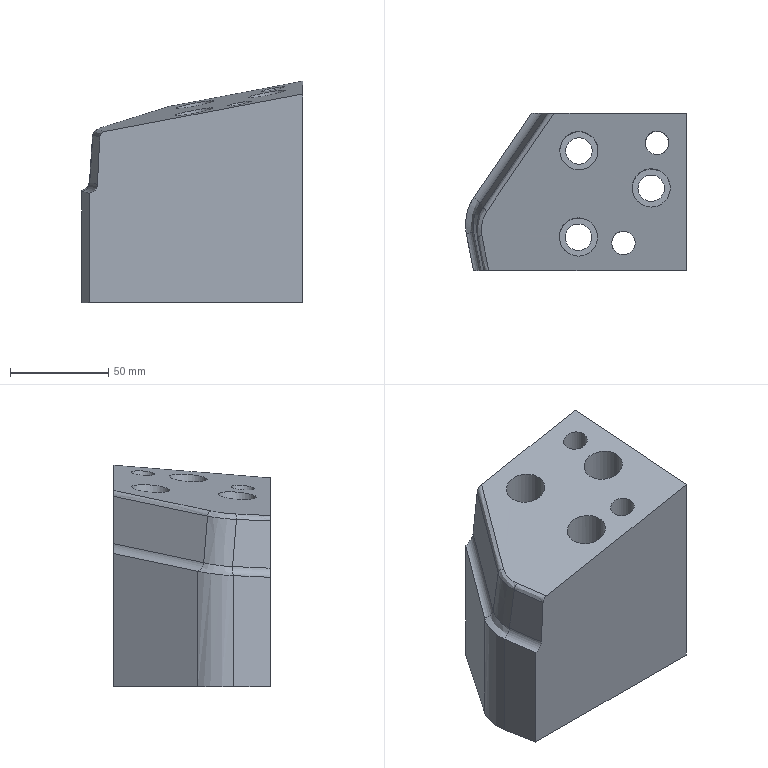Part | NX | features solid 2 | 1 solid | 28 faces | box 112.653 x 80 x 112.905 mm | volume 689812 mm3 | cylinder 10 | spline 9 | plane 9 | commonest cylinder face diameters 13.5 x3 19.5 x3 10 x2 12 x2
STEP:
#1=CARTESIAN_POINT('',(910.176,4.689,67.517));
#2=VERTEX_POINT('',#1);
#3=CARTESIAN_POINT('',(904.312,-0.5268,65.98));
#4=CARTESIAN_POINT('',(911.039,4.097,67.632));
#5=CARTESIAN_POINT('',(912.591,12.271,68.592));
#6=CARTESIAN_POINT('',(907.787,19.138,68.239));
#7=CARTESIAN_POINT('',(899.676,20.525,66.813));
#8=CARTESIAN_POINT('',(892.968,15.903,65.165));
#9=CARTESIAN_POINT('',(891.404,7.747,64.204));
#10=CARTESIAN_POINT('',(896.213,0.8606,64.556));
#11=CARTESIAN_POINT('',(904.312,-0.5268,65.98));
#12=CARTESIAN_POINT('',(911.039,4.097,67.632));
#13=CARTESIAN_POINT('',(912.591,12.271,68.592));
#14=B_SPLINE_CURVE_WITH_KNOTS('',3,(#3,#4,#5,#6,#7,#8,#9,#10,#11,#12,#13),.UNSPECIFIED.,.T.,.F.,(1,1,1,1,1,1,1,1,1,1,1,1,1,1,1),(-0.0231,-0.0154,-0.007701,0.,0.007701,0.0154,0.0231,0.0308,0.03851,0.04621,0.05391,0.06161,0.06931,0.07701,0.08471),.UNSPECIFIED.);
#15=EDGE_CURVE('',#2,#2,#14,.T.);
#16=ORIENTED_EDGE('',*,*,#15,.F.);
#17=EDGE_LOOP('',(#16));
#18=FACE_BOUND('',#17,.T.);
#19=CARTESIAN_POINT('',(874.601,-16.091,59.076));
#20=VERTEX_POINT('',#19);
#21=CARTESIAN_POINT('',(871.629,-23.43,57.915));
#22=CARTESIAN_POINT('',(875.665,-16.236,59.267));
#23=CARTESIAN_POINT('',(873.318,-8.171,59.478));
#24=CARTESIAN_POINT('',(866.002,-4.266,58.407));
#25=CARTESIAN_POINT('',(858.186,-6.577,56.737));
#26=CARTESIAN_POINT('',(854.166,-13.76,55.389));
#27=CARTESIAN_POINT('',(856.494,-21.817,55.175));
#28=CARTESIAN_POINT('',(863.825,-25.735,56.247));
#29=CARTESIAN_POINT('',(871.629,-23.43,57.915));
#30=CARTESIAN_POINT('',(875.665,-16.236,59.267));
#31=CARTESIAN_POINT('',(873.318,-8.171,59.478));
#32=B_SPLINE_CURVE_WITH_KNOTS('',3,(#21,#22,#23,#24,#25,#26,#27,#28,#29,#30,#31),.UNSPECIFIED.,.T.,.F.,(1,1,1,1,1,1,1,1,1,1,1,1,1,1,1),(-0.02311,-0.0154,-0.007702,0.,0.007702,0.0154,0.02311,0.03081,0.03851,0.04621,0.05392,0.06162,0.06932,0.07702,0.08472),.UNSPECIFIED.);
#33=EDGE_CURVE('',#20,#20,#32,.T.);
#34=ORIENTED_EDGE('',*,*,#33,.F.);
#35=EDGE_LOOP('',(#34));
#36=FACE_BOUND('',#35,.T.);
#37=CARTESIAN_POINT('',(874.42,25.901,62.459));
#38=VERTEX_POINT('',#37);
#39=CARTESIAN_POINT('',(870.01,19.371,61.091));
#40=CARTESIAN_POINT('',(875.417,25.536,62.619));
#41=CARTESIAN_POINT('',(874.842,33.891,63.19));
#42=CARTESIAN_POINT('',(868.479,39.284,62.421));
#43=CARTESIAN_POINT('',(860.329,38.624,60.821));
#44=CARTESIAN_POINT('',(854.941,32.466,59.298));
#45=CARTESIAN_POINT('',(855.498,24.125,58.725));
#46=CARTESIAN_POINT('',(861.874,18.715,59.494));
#47=CARTESIAN_POINT('',(870.01,19.371,61.091));
#48=CARTESIAN_POINT('',(875.417,25.536,62.619));
#49=CARTESIAN_POINT('',(874.842,33.891,63.19));
#50=B_SPLINE_CURVE_WITH_KNOTS('',3,(#39,#40,#41,#42,#43,#44,#45,#46,#47,#48,#49),.UNSPECIFIED.,.T.,.F.,(1,1,1,1,1,1,1,1,1,1,1,1,1,1,1),(-0.02311,-0.0154,-0.007702,0.,0.007702,0.0154,0.02311,0.03081,0.03851,0.04621,0.05391,0.06162,0.06932,0.07702,0.08472),.UNSPECIFIED.);
#51=EDGE_CURVE('',#38,#38,#50,.T.);
#52=ORIENTED_EDGE('',*,*,#51,.F.);
#53=EDGE_LOOP('',(#52));
#54=FACE_BOUND('',#53,.T.);
#55=CARTESIAN_POINT('',(900.381,36.794,68.271));
#56=VERTEX_POINT('',#55);
#57=CARTESIAN_POINT('',(904.331,39.565,69.246));
#58=CARTESIAN_POINT('',(899.898,37.213,68.213));
#59=CARTESIAN_POINT('',(898.365,32.347,67.527));
#60=CARTESIAN_POINT('',(900.8,27.795,67.618));
#61=CARTESIAN_POINT('',(905.676,26.363,68.427));
#62=CARTESIAN_POINT('',(910.098,28.715,69.457));
#63=CARTESIAN_POINT('',(911.636,33.57,70.144));
#64=CARTESIAN_POINT('',(909.201,38.133,70.053));
#65=CARTESIAN_POINT('',(904.331,39.565,69.246));
#66=CARTESIAN_POINT('',(899.898,37.213,68.213));
#67=CARTESIAN_POINT('',(898.365,32.347,67.527));
#68=B_SPLINE_CURVE_WITH_KNOTS('',3,(#57,#58,#59,#60,#61,#62,#63,#64,#65,#66,#67),.UNSPECIFIED.,.T.,.F.,(1,1,1,1,1,1,1,1,1,1,1,1,1,1,1),(-0.01422,-0.009478,-0.004739,0.,0.004739,0.009478,0.01422,0.01896,0.02369,0.02843,0.03317,0.03791,0.04265,0.04739,0.05213),.UNSPECIFIED.);
#69=EDGE_CURVE('',#56,#56,#68,.T.);
#70=ORIENTED_EDGE('',*,*,#69,.F.);
#71=EDGE_LOOP('',(#70));
#72=FACE_BOUND('',#71,.T.);
#73=CARTESIAN_POINT('',(818.332,-1.794,49.565));
#74=VERTEX_POINT('',#73);
#75=CARTESIAN_POINT('',(815.743,-14.303,48.056));
#76=VERTEX_POINT('',#75);
#77=CARTESIAN_POINT('',(818.332,-1.794,49.565));
#78=CARTESIAN_POINT('',(815.864,-5.396,48.803));
#79=CARTESIAN_POINT('',(814.905,-9.954,48.251));
#80=CARTESIAN_POINT('',(815.743,-14.303,48.056));
#81=B_SPLINE_CURVE_WITH_KNOTS('',3,(#77,#78,#79,#80),.UNSPECIFIED.,.F.,.F.,(4,4),(0.,0.01319),.UNSPECIFIED.);
#82=EDGE_CURVE('',#74,#76,#81,.T.);
#83=ORIENTED_EDGE('',*,*,#82,.T.);
#84=CARTESIAN_POINT('',(819.154,-32.,47.263));
#85=VERTEX_POINT('',#84);
#86=CARTESIAN_POINT('',(815.743,-14.303,48.056));
#87=CARTESIAN_POINT('',(816.88,-20.202,47.791));
#88=CARTESIAN_POINT('',(818.017,-26.101,47.527));
#89=CARTESIAN_POINT('',(819.154,-32.,47.263));
#90=B_SPLINE_CURVE_WITH_KNOTS('',3,(#86,#87,#88,#89),.UNSPECIFIED.,.F.,.F.,(4,4),(0.,0.01804),.UNSPECIFIED.);
#91=EDGE_CURVE('',#76,#85,#90,.T.);
#92=ORIENTED_EDGE('',*,*,#91,.T.);
#93=CARTESIAN_POINT('',(920.,-32.,66.395));
#94=VERTEX_POINT('',#93);
#95=CARTESIAN_POINT('',(819.154,-32.,47.263));
#96=CARTESIAN_POINT('',(852.769,-32.,53.64));
#97=CARTESIAN_POINT('',(886.385,-32.,60.017));
#98=CARTESIAN_POINT('',(920.,-32.,66.395));
#99=B_SPLINE_CURVE_WITH_KNOTS('',3,(#95,#96,#97,#98),.UNSPECIFIED.,.F.,.F.,(4,4),(0.,0.1026),.UNSPECIFIED.);
#100=EDGE_CURVE('',#85,#94,#99,.T.);
#101=ORIENTED_EDGE('',*,*,#100,.T.);
#102=CARTESIAN_POINT('',(920.,48.,72.905));
#103=VERTEX_POINT('',#102);
#104=CARTESIAN_POINT('',(920.,-32.,66.395));
#105=CARTESIAN_POINT('',(920.,-5.333,68.565));
#106=CARTESIAN_POINT('',(920.,21.333,70.735));
#107=CARTESIAN_POINT('',(920.,48.,72.905));
#108=B_SPLINE_CURVE_WITH_KNOTS('',3,(#104,#105,#106,#107),.UNSPECIFIED.,.F.,.F.,(4,4),(0.,0.08026),.UNSPECIFIED.);
#109=EDGE_CURVE('',#94,#103,#108,.T.);
#110=ORIENTED_EDGE('',*,*,#109,.T.);
#111=CARTESIAN_POINT('',(852.448,48.,60.089));
#112=VERTEX_POINT('',#111);
#113=CARTESIAN_POINT('',(852.448,48.,60.089));
#114=CARTESIAN_POINT('',(874.965,48.,64.361));
#115=CARTESIAN_POINT('',(897.483,48.,68.633));
#116=CARTESIAN_POINT('',(920.,48.,72.905));
#117=B_SPLINE_CURVE_WITH_KNOTS('',3,(#113,#114,#115,#116),.UNSPECIFIED.,.F.,.F.,(4,4),(0.,0.06876),.UNSPECIFIED.);
#118=EDGE_CURVE('',#112,#103,#117,.T.);
#119=ORIENTED_EDGE('',*,*,#118,.F.);
#120=CARTESIAN_POINT('',(852.448,48.,60.089));
#121=CARTESIAN_POINT('',(841.076,31.402,56.581));
#122=CARTESIAN_POINT('',(829.704,14.804,53.073));
#123=CARTESIAN_POINT('',(818.332,-1.794,49.565));
#124=B_SPLINE_CURVE_WITH_KNOTS('',3,(#120,#121,#122,#123),.UNSPECIFIED.,.F.,.F.,(4,4),(0.0001037,0.06137),.UNSPECIFIED.);
#125=EDGE_CURVE('',#112,#74,#124,.T.);
#126=ORIENTED_EDGE('',*,*,#125,.T.);
#127=EDGE_LOOP('',(#83,#92,#101,#110,#119,#126));
#128=FACE_BOUND('',#127,.T.);
#129=CARTESIAN_POINT('',(882.556,-15.206,60.658));
#130=VERTEX_POINT('',#129);
#131=CARTESIAN_POINT('',(885.863,-11.678,61.572));
#132=CARTESIAN_POINT('',(881.991,-14.889,60.576));
#133=CARTESIAN_POINT('',(881.506,-20.,60.068));
#134=CARTESIAN_POINT('',(884.84,-23.925,60.381));
#135=CARTESIAN_POINT('',(889.875,-24.32,61.305));
#136=CARTESIAN_POINT('',(893.735,-21.111,62.298));
#137=CARTESIAN_POINT('',(894.229,-16.011,62.807));
#138=CARTESIAN_POINT('',(890.89,-12.074,62.494));
#139=CARTESIAN_POINT('',(885.863,-11.678,61.572));
#140=CARTESIAN_POINT('',(881.991,-14.889,60.576));
#141=CARTESIAN_POINT('',(881.506,-20.,60.068));
#142=B_SPLINE_CURVE_WITH_KNOTS('',3,(#131,#132,#133,#134,#135,#136,#137,#138,#139,#140,#141),.UNSPECIFIED.,.T.,.F.,(1,1,1,1,1,1,1,1,1,1,1,1,1,1,1),(-0.01422,-0.009479,-0.004739,0.,0.004739,0.009479,0.01422,0.01896,0.0237,0.02844,0.03318,0.03791,0.04265,0.04739,0.05213),.UNSPECIFIED.);
#143=EDGE_CURVE('',#130,#130,#142,.T.);
#144=ORIENTED_EDGE('',*,*,#143,.F.);
#145=EDGE_LOOP('',(#144));
#146=FACE_BOUND('',#145,.T.);
#147=CARTESIAN_POINT('',(920.361,48.485,73.013));
#148=CARTESIAN_POINT('',(919.989,-34.505,66.189));
#149=CARTESIAN_POINT('',(900.884,48.874,69.349));
#150=CARTESIAN_POINT('',(900.511,-34.116,62.525));
#151=CARTESIAN_POINT('',(894.725,48.997,68.191));
#152=CARTESIAN_POINT('',(894.352,-33.993,61.367));
#153=CARTESIAN_POINT('',(815.085,50.586,53.211));
#154=CARTESIAN_POINT('',(814.713,-32.403,46.387));
#155=B_SPLINE_SURFACE_WITH_KNOTS('',1,1,((#147,#148),(#149,#150),(#151,#152),(#153,#154)),.PLANE_SURF.,.F.,.F.,.F.,(2,1,1,2),(2,2),(-0.109,-0.02619,0.,0.3387),(0.4195,0.7113),.PIECEWISE_BEZIER_KNOTS.);
#156=ADVANCED_FACE('',(#18,#36,#54,#72,#128,#146),#155,.T.);
#157=CARTESIAN_POINT('',(871.662,-15.,-40.));
#158=VERTEX_POINT('',#157);
#159=CARTESIAN_POINT('',(864.912,-15.,-40.));
#160=DIRECTION('',(0.,0.,1.));
#161=DIRECTION('',(1.,0.,0.));
#162=AXIS2_PLACEMENT_3D('',#159,#160,#161);
#163=CIRCLE('',#162,6.75);
#164=EDGE_CURVE('',#158,#158,#163,.F.);
#165=ORIENTED_EDGE('',*,*,#164,.F.);
#166=EDGE_LOOP('',(#165));
#167=FACE_BOUND('',#166,.T.);
#168=CARTESIAN_POINT('',(911.,32.964,-40.));
#169=VERTEX_POINT('',#168);
#170=CARTESIAN_POINT('',(905.,32.964,-40.));
#171=DIRECTION('',(0.,0.,1.));
#172=DIRECTION('',(1.,0.,0.));
#173=AXIS2_PLACEMENT_3D('',#170,#171,#172);
#174=CIRCLE('',#173,6.);
#175=EDGE_CURVE('',#169,#169,#174,.T.);
#176=ORIENTED_EDGE('',*,*,#175,.T.);
#177=EDGE_LOOP('',(#176));
#178=FACE_BOUND('',#177,.T.);
#179=CARTESIAN_POINT('',(908.75,10.,-40.));
#180=VERTEX_POINT('',#179);
#181=CARTESIAN_POINT('',(902.,10.,-40.));
#182=DIRECTION('',(0.,0.,1.));
#183=DIRECTION('',(1.,0.,0.));
#184=AXIS2_PLACEMENT_3D('',#181,#182,#183);
#185=CIRCLE('',#184,6.75);
#186=EDGE_CURVE('',#180,#180,#185,.T.);
#187=ORIENTED_EDGE('',*,*,#186,.T.);
#188=EDGE_LOOP('',(#187));
#189=FACE_BOUND('',#188,.T.);
#190=CARTESIAN_POINT('',(920.,-32.,-40.));
#191=VERTEX_POINT('',#190);
#192=CARTESIAN_POINT('',(920.,48.,-40.));
#193=VERTEX_POINT('',#192);
#194=CARTESIAN_POINT('',(920.,8.,-40.));
#195=DIRECTION('',(0.,-1.,0.));
#196=VECTOR('',#195,1000.);
#197=LINE('',#194,#196);
#198=EDGE_CURVE('',#191,#193,#197,.F.);
#199=ORIENTED_EDGE('',*,*,#198,.F.);
#200=CARTESIAN_POINT('',(811.412,-32.,-40.));
#201=VERTEX_POINT('',#200);
#202=CARTESIAN_POINT('',(915.5,-32.,-40.));
#203=DIRECTION('',(-1.,0.,0.));
#204=VECTOR('',#203,1000.);
#205=LINE('',#202,#204);
#206=EDGE_CURVE('',#201,#191,#205,.F.);
#207=ORIENTED_EDGE('',*,*,#206,.F.);
#208=CARTESIAN_POINT('',(807.792,-13.215,-40.));
#209=VERTEX_POINT('',#208);
#210=CARTESIAN_POINT('',(811.353,-31.695,-40.));
#211=DIRECTION('',(-0.1892,0.9819,0.));
#212=VECTOR('',#211,1000.);
#213=LINE('',#210,#212);
#214=EDGE_CURVE('',#201,#209,#213,.T.);
#215=ORIENTED_EDGE('',*,*,#214,.T.);
#216=CARTESIAN_POINT('',(811.599,5.18,-40.));
#217=VERTEX_POINT('',#216);
#218=CARTESIAN_POINT('',(807.792,-13.215,-40.));
#219=CARTESIAN_POINT('',(806.568,-6.861,-40.));
#220=CARTESIAN_POINT('',(807.942,-0.1588,-40.));
#221=CARTESIAN_POINT('',(811.599,5.18,-40.));
#222=B_SPLINE_CURVE_WITH_KNOTS('',3,(#218,#219,#220,#221),.UNSPECIFIED.,.F.,.F.,(4,4),(0.,0.01932),.UNSPECIFIED.);
#223=EDGE_CURVE('',#209,#217,#222,.T.);
#224=ORIENTED_EDGE('',*,*,#223,.T.);
#225=CARTESIAN_POINT('',(840.937,48.,-40.));
#226=VERTEX_POINT('',#225);
#227=CARTESIAN_POINT('',(811.599,5.18,-40.));
#228=DIRECTION('',(0.5652,0.8249,0.));
#229=VECTOR('',#228,1000.);
#230=LINE('',#227,#229);
#231=EDGE_CURVE('',#217,#226,#230,.T.);
#232=ORIENTED_EDGE('',*,*,#231,.T.);
#233=CARTESIAN_POINT('',(915.5,48.,-40.));
#234=DIRECTION('',(1.,0.,0.));
#235=VECTOR('',#234,1000.);
#236=LINE('',#233,#235);
#237=EDGE_CURVE('',#226,#193,#236,.T.);
#238=ORIENTED_EDGE('',*,*,#237,.T.);
#239=EDGE_LOOP('',(#199,#207,#215,#224,#232,#238));
#240=FACE_BOUND('',#239,.T.);
#241=CARTESIAN_POINT('',(893.865,-18.,-40.));
#242=VERTEX_POINT('',#241);
#243=CARTESIAN_POINT('',(887.865,-18.,-40.));
#244=DIRECTION('',(0.,0.,1.));
#245=DIRECTION('',(1.,0.,0.));
#246=AXIS2_PLACEMENT_3D('',#243,#244,#245);
#247=CIRCLE('',#246,6.);
#248=EDGE_CURVE('',#242,#242,#247,.T.);
#249=ORIENTED_EDGE('',*,*,#248,.T.);
#250=EDGE_LOOP('',(#249));
#251=FACE_BOUND('',#250,.T.);
#252=CARTESIAN_POINT('',(871.925,29.,-40.));
#253=VERTEX_POINT('',#252);
#254=CARTESIAN_POINT('',(865.175,29.,-40.));
#255=DIRECTION('',(0.,0.,1.));
#256=DIRECTION('',(1.,0.,0.));
#257=AXIS2_PLACEMENT_3D('',#254,#255,#256);
#258=CIRCLE('',#257,6.75);
#259=EDGE_CURVE('',#253,#253,#258,.F.);
#260=ORIENTED_EDGE('',*,*,#259,.F.);
#261=EDGE_LOOP('',(#260));
#262=FACE_BOUND('',#261,.T.);
#263=CARTESIAN_POINT('',(878.5,8.,-40.));
#264=DIRECTION('',(0.,0.,1.));
#265=DIRECTION('',(0.,-1.,0.));
#266=AXIS2_PLACEMENT_3D('',#263,#264,#265);
#267=PLANE('',#266);
#268=ADVANCED_FACE('',(#167,#178,#189,#240,#251,#262),#267,.F.);
#269=CARTESIAN_POINT('',(811.599,5.18,18.855));
#270=VERTEX_POINT('',#269);
#271=CARTESIAN_POINT('',(811.599,5.18,100.));
#272=DIRECTION('',(0.,0.,-1.));
#273=VECTOR('',#272,1000.);
#274=LINE('',#271,#273);
#275=EDGE_CURVE('',#270,#217,#274,.T.);
#276=ORIENTED_EDGE('',*,*,#275,.F.);
#277=CARTESIAN_POINT('',(840.937,48.,27.905));
#278=VERTEX_POINT('',#277);
#279=CARTESIAN_POINT('',(811.599,5.18,18.855));
#280=CARTESIAN_POINT('',(821.379,19.454,21.872));
#281=CARTESIAN_POINT('',(831.158,33.727,24.889));
#282=CARTESIAN_POINT('',(840.937,48.,27.905));
#283=B_SPLINE_CURVE_WITH_KNOTS('',3,(#279,#280,#281,#282),.UNSPECIFIED.,.F.,.F.,(4,4),(0.,0.998),.UNSPECIFIED.);
#284=EDGE_CURVE('',#270,#278,#283,.T.);
#285=ORIENTED_EDGE('',*,*,#284,.T.);
#286=CARTESIAN_POINT('',(840.937,48.,100.));
#287=DIRECTION('',(0.,0.,-1.));
#288=VECTOR('',#287,1000.);
#289=LINE('',#286,#288);
#290=EDGE_CURVE('',#278,#226,#289,.T.);
#291=ORIENTED_EDGE('',*,*,#290,.T.);
#292=ORIENTED_EDGE('',*,*,#231,.F.);
#293=EDGE_LOOP('',(#276,#285,#291,#292));
#294=FACE_BOUND('',#293,.T.);
#295=CARTESIAN_POINT('',(811.599,5.18,100.));
#296=DIRECTION('',(-0.8249,0.5652,0.));
#297=DIRECTION('',(-0.5652,-0.8249,0.));
#298=AXIS2_PLACEMENT_3D('',#295,#296,#297);
#299=PLANE('',#298);
#300=ADVANCED_FACE('',(#294),#299,.T.);
#301=CARTESIAN_POINT('',(807.792,-13.215,16.636));
#302=VERTEX_POINT('',#301);
#303=CARTESIAN_POINT('',(807.792,-13.215,100.));
#304=DIRECTION('',(0.,0.,-1.));
#305=VECTOR('',#304,1000.);
#306=LINE('',#303,#305);
#307=EDGE_CURVE('',#302,#209,#306,.T.);
#308=ORIENTED_EDGE('',*,*,#307,.F.);
#309=CARTESIAN_POINT('',(807.792,-13.215,16.636));
#310=CARTESIAN_POINT('',(807.495,-11.672,16.705));
#311=CARTESIAN_POINT('',(807.267,-9.272,16.857));
#312=CARTESIAN_POINT('',(807.43,-6.053,17.15));
#313=CARTESIAN_POINT('',(807.829,-3.53,17.431));
#314=CARTESIAN_POINT('',(808.377,-1.426,17.706));
#315=CARTESIAN_POINT('',(809.45,1.568,18.154));
#316=CARTESIAN_POINT('',(810.629,3.763,18.556));
#317=CARTESIAN_POINT('',(811.599,5.18,18.855));
#318=B_SPLINE_CURVE_WITH_KNOTS('',3,(#309,#310,#311,#312,#313,#314,#315,#316,#317),.UNSPECIFIED.,.F.,.F.,(4,1,1,1,1,1,4),(0.,0.25,0.375,0.5,0.625,0.75,1.),.UNSPECIFIED.);
#319=EDGE_CURVE('',#270,#302,#318,.F.);
#320=ORIENTED_EDGE('',*,*,#319,.F.);
#321=ORIENTED_EDGE('',*,*,#275,.T.);
#322=ORIENTED_EDGE('',*,*,#223,.F.);
#323=EDGE_LOOP('',(#308,#320,#321,#322));
#324=FACE_BOUND('',#323,.T.);
#325=CARTESIAN_POINT('',(807.792,-13.215,19.208));
#326=CARTESIAN_POINT('',(807.792,-13.215,-40.));
#327=CARTESIAN_POINT('',(807.18,-10.038,19.208));
#328=CARTESIAN_POINT('',(807.18,-10.038,-40.));
#329=CARTESIAN_POINT('',(807.22,-3.453,19.208));
#330=CARTESIAN_POINT('',(807.22,-3.453,-40.));
#331=CARTESIAN_POINT('',(809.797,2.549,19.208));
#332=CARTESIAN_POINT('',(809.797,2.549,-40.));
#333=CARTESIAN_POINT('',(811.599,5.18,19.208));
#334=CARTESIAN_POINT('',(811.599,5.18,-40.));
#335=B_SPLINE_SURFACE_WITH_KNOTS('',3,1,((#325,#326),(#327,#328),(#329,#330),(#331,#332),(#333,#334)),.SURF_OF_LINEAR_EXTRUSION.,.F.,.F.,.F.,(4,1,4),(2,2),(0.,0.5,1.),(0.,1.),.UNSPECIFIED.);
#336=ADVANCED_FACE('',(#324),#335,.T.);
#337=CARTESIAN_POINT('',(811.412,-32.,15.794));
#338=VERTEX_POINT('',#337);
#339=CARTESIAN_POINT('',(811.412,-32.,100.));
#340=DIRECTION('',(0.,0.,1.));
#341=VECTOR('',#340,1000.);
#342=LINE('',#339,#341);
#343=EDGE_CURVE('',#338,#201,#342,.F.);
#344=ORIENTED_EDGE('',*,*,#343,.F.);
#345=CARTESIAN_POINT('',(811.412,-32.,15.794));
#346=CARTESIAN_POINT('',(810.206,-25.738,16.075));
#347=CARTESIAN_POINT('',(808.999,-19.477,16.355));
#348=CARTESIAN_POINT('',(807.792,-13.215,16.636));
#349=B_SPLINE_CURVE_WITH_KNOTS('',3,(#345,#346,#347,#348),.UNSPECIFIED.,.F.,.F.,(4,4),(-0.01648,1.),.UNSPECIFIED.);
#350=EDGE_CURVE('',#338,#302,#349,.T.);
#351=ORIENTED_EDGE('',*,*,#350,.T.);
#352=ORIENTED_EDGE('',*,*,#307,.T.);
#353=ORIENTED_EDGE('',*,*,#214,.F.);
#354=EDGE_LOOP('',(#344,#351,#352,#353));
#355=FACE_BOUND('',#354,.T.);
#356=CARTESIAN_POINT('',(811.353,-31.695,100.));
#357=DIRECTION('',(-0.9819,-0.1892,0.));
#358=DIRECTION('',(0.1892,-0.9819,0.));
#359=AXIS2_PLACEMENT_3D('',#356,#357,#358);
#360=PLANE('',#359);
#361=ADVANCED_FACE('',(#355),#360,.T.);
#362=CARTESIAN_POINT('',(849.224,48.,57.055));
#363=VERTEX_POINT('',#362);
#364=CARTESIAN_POINT('',(846.311,48.,32.963));
#365=VERTEX_POINT('',#364);
#366=CARTESIAN_POINT('',(849.224,48.,57.055));
#367=CARTESIAN_POINT('',(848.253,48.,49.024));
#368=CARTESIAN_POINT('',(847.282,48.,40.994));
#369=CARTESIAN_POINT('',(846.311,48.,32.963));
#370=B_SPLINE_CURVE_WITH_KNOTS('',3,(#366,#367,#368,#369),.UNSPECIFIED.,.F.,.F.,(4,4),(0.,0.02427),.UNSPECIFIED.);
#371=EDGE_CURVE('',#363,#365,#370,.T.);
#372=ORIENTED_EDGE('',*,*,#371,.F.);
#373=CARTESIAN_POINT('',(849.224,48.,57.055));
#374=CARTESIAN_POINT('',(849.32,48.,57.845));
#375=CARTESIAN_POINT('',(850.207,48.,59.255));
#376=CARTESIAN_POINT('',(851.67,48.,59.941));
#377=CARTESIAN_POINT('',(852.448,48.,60.089));
#378=B_SPLINE_CURVE_WITH_KNOTS('',3,(#373,#374,#375,#376,#377),.UNSPECIFIED.,.F.,.F.,(4,1,4),(0.,0.002349,0.004697),.UNSPECIFIED.);
#379=EDGE_CURVE('',#363,#112,#378,.T.);
#380=ORIENTED_EDGE('',*,*,#379,.T.);
#381=ORIENTED_EDGE('',*,*,#118,.T.);
#382=CARTESIAN_POINT('',(920.,48.,-47.5));
#383=DIRECTION('',(0.,0.,1.));
#384=VECTOR('',#383,1000.);
#385=LINE('',#382,#384);
#386=EDGE_CURVE('',#103,#193,#385,.F.);
#387=ORIENTED_EDGE('',*,*,#386,.T.);
#388=ORIENTED_EDGE('',*,*,#237,.F.);
#389=ORIENTED_EDGE('',*,*,#290,.F.);
#390=CARTESIAN_POINT('',(840.281,48.,32.886));
#391=DIRECTION('',(0.,1.,0.));
#392=DIRECTION('',(-0.9556,0.,-0.2948));
#393=AXIS2_PLACEMENT_3D('',#390,#391,#392);
#394=ELLIPSE('',#393,6.152,5.);
#395=EDGE_CURVE('',#278,#365,#394,.F.);
#396=ORIENTED_EDGE('',*,*,#395,.T.);
#397=EDGE_LOOP('',(#372,#380,#381,#387,#388,#389,#396));
#398=FACE_BOUND('',#397,.T.);
#399=CARTESIAN_POINT('',(915.5,48.,-47.5));
#400=DIRECTION('',(0.,1.,0.));
#401=DIRECTION('',(1.,0.,0.));
#402=AXIS2_PLACEMENT_3D('',#399,#400,#401);
#403=PLANE('',#402);
#404=ADVANCED_FACE('',(#398),#403,.T.);
#405=ORIENTED_EDGE('',*,*,#198,.T.);
#406=ORIENTED_EDGE('',*,*,#386,.F.);
#407=ORIENTED_EDGE('',*,*,#109,.F.);
#408=CARTESIAN_POINT('',(920.,-32.,-47.5));
#409=DIRECTION('',(0.,0.,-1.));
#410=VECTOR('',#409,1000.);
#411=LINE('',#408,#410);
#412=EDGE_CURVE('',#94,#191,#411,.T.);
#413=ORIENTED_EDGE('',*,*,#412,.T.);
#414=EDGE_LOOP('',(#405,#406,#407,#413));
#415=FACE_BOUND('',#414,.T.);
#416=CARTESIAN_POINT('',(920.,-31.695,100.));
#417=DIRECTION('',(-1.,0.,0.));
#418=DIRECTION('',(0.,0.,1.));
#419=AXIS2_PLACEMENT_3D('',#416,#417,#418);
#420=PLANE('',#419);
#421=ADVANCED_FACE('',(#415),#420,.F.);
#422=ORIENTED_EDGE('',*,*,#100,.F.);
#423=CARTESIAN_POINT('',(816.706,-32.,44.488));
#424=VERTEX_POINT('',#423);
#425=CARTESIAN_POINT('',(819.154,-32.,47.263));
#426=CARTESIAN_POINT('',(817.835,-32.,47.012));
#427=CARTESIAN_POINT('',(816.773,-32.,45.829));
#428=CARTESIAN_POINT('',(816.706,-32.,44.488));
#429=B_SPLINE_CURVE_WITH_KNOTS('',3,(#425,#426,#427,#428),.UNSPECIFIED.,.F.,.F.,(4,4),(0.,0.00397),.UNSPECIFIED.);
#430=EDGE_CURVE('',#85,#424,#429,.T.);
#431=ORIENTED_EDGE('',*,*,#430,.T.);
#432=CARTESIAN_POINT('',(815.492,-32.,20.419));
#433=VERTEX_POINT('',#432);
#434=CARTESIAN_POINT('',(816.706,-32.,44.488));
#435=CARTESIAN_POINT('',(816.301,-32.,36.465));
#436=CARTESIAN_POINT('',(815.897,-32.,28.442));
#437=CARTESIAN_POINT('',(815.492,-32.,20.419));
#438=B_SPLINE_CURVE_WITH_KNOTS('',3,(#434,#435,#436,#437),.UNSPECIFIED.,.F.,.F.,(4,4),(0.,0.0241),.UNSPECIFIED.);
#439=EDGE_CURVE('',#424,#433,#438,.T.);
#440=ORIENTED_EDGE('',*,*,#439,.T.);
#441=CARTESIAN_POINT('',(810.406,-32.,20.708));
#442=DIRECTION('',(0.,-1.,0.));
#443=DIRECTION('',(0.974,0.,-0.2265));
#444=AXIS2_PLACEMENT_3D('',#441,#442,#443);
#445=ELLIPSE('',#444,5.097,5.);
#446=EDGE_CURVE('',#338,#433,#445,.T.);
#447=ORIENTED_EDGE('',*,*,#446,.F.);
#448=ORIENTED_EDGE('',*,*,#343,.T.);
#449=ORIENTED_EDGE('',*,*,#206,.T.);
#450=ORIENTED_EDGE('',*,*,#412,.F.);
#451=EDGE_LOOP('',(#422,#431,#440,#447,#448,#449,#450));
#452=FACE_BOUND('',#451,.T.);
#453=CARTESIAN_POINT('',(915.5,-32.,-47.5));
#454=DIRECTION('',(0.,-1.,0.));
#455=DIRECTION('',(-1.,0.,0.));
#456=AXIS2_PLACEMENT_3D('',#453,#454,#455);
#457=PLANE('',#456);
#458=ADVANCED_FACE('',(#452),#457,.T.);
#459=ORIENTED_EDGE('',*,*,#350,.F.);
#460=ORIENTED_EDGE('',*,*,#446,.T.);
#461=CARTESIAN_POINT('',(815.115,-30.041,20.506));
#462=VERTEX_POINT('',#461);
#463=CARTESIAN_POINT('',(815.115,-30.041,20.506));
#464=CARTESIAN_POINT('',(815.24,-30.694,20.477));
#465=CARTESIAN_POINT('',(815.366,-31.347,20.448));
#466=CARTESIAN_POINT('',(815.492,-32.,20.419));
#467=B_SPLINE_CURVE_WITH_KNOTS('',3,(#463,#464,#465,#466),.UNSPECIFIED.,.F.,.F.,(4,4),(0.,0.1994),.UNSPECIFIED.);
#468=EDGE_CURVE('',#462,#433,#467,.T.);
#469=ORIENTED_EDGE('',*,*,#468,.F.);
#470=CARTESIAN_POINT('',(815.095,-29.937,20.511));
#471=VERTEX_POINT('',#470);
#472=CARTESIAN_POINT('',(815.115,-30.041,20.506));
#473=CARTESIAN_POINT('',(815.108,-30.007,20.508));
#474=CARTESIAN_POINT('',(815.101,-29.972,20.509));
#475=CARTESIAN_POINT('',(815.095,-29.937,20.511));
#476=B_SPLINE_CURVE_WITH_KNOTS('',3,(#472,#473,#474,#475),.UNSPECIFIED.,.F.,.F.,(4,4),(0.,1.),.UNSPECIFIED.);
#477=EDGE_CURVE('',#471,#462,#476,.F.);
#478=ORIENTED_EDGE('',*,*,#477,.F.);
#479=CARTESIAN_POINT('',(811.765,-12.658,21.285));
#480=VERTEX_POINT('',#479);
#481=CARTESIAN_POINT('',(811.765,-12.658,21.285));
#482=CARTESIAN_POINT('',(812.875,-18.418,21.027));
#483=CARTESIAN_POINT('',(813.985,-24.178,20.769));
#484=CARTESIAN_POINT('',(815.095,-29.937,20.511));
#485=B_SPLINE_CURVE_WITH_KNOTS('',3,(#481,#482,#483,#484),.UNSPECIFIED.,.F.,.F.,(4,4),(0.,1.),.UNSPECIFIED.);
#486=EDGE_CURVE('',#480,#471,#485,.T.);
#487=ORIENTED_EDGE('',*,*,#486,.F.);
#488=CARTESIAN_POINT('',(807.792,-13.215,16.636));
#489=CARTESIAN_POINT('',(808.855,-13.02,16.853));
#490=CARTESIAN_POINT('',(810.836,-12.691,18.028));
#491=CARTESIAN_POINT('',(811.702,-12.621,20.186));
#492=CARTESIAN_POINT('',(811.765,-12.658,21.285));
#493=B_SPLINE_CURVE_WITH_KNOTS('',3,(#488,#489,#490,#491,#492),.UNSPECIFIED.,.F.,.F.,(4,1,4),(0.,0.5,1.),.UNSPECIFIED.);
#494=EDGE_CURVE('',#302,#480,#493,.T.);
#495=ORIENTED_EDGE('',*,*,#494,.F.);
#496=EDGE_LOOP('',(#459,#460,#469,#478,#487,#495));
#497=FACE_BOUND('',#496,.T.);
#498=CARTESIAN_POINT('',(795.674,44.457,24.135));
#499=DIRECTION('',(0.189,-0.981,-0.04397));
#500=DIRECTION('',(0.9803,0.1911,-0.04943));
#501=AXIS2_PLACEMENT_3D('',#498,#499,#500);
#502=CYLINDRICAL_SURFACE('',#501,5.);
#503=ADVANCED_FACE('',(#497),#502,.F.);
#504=ORIENTED_EDGE('',*,*,#439,.F.);
#505=CARTESIAN_POINT('',(813.36,-14.637,45.266));
#506=VERTEX_POINT('',#505);
#507=CARTESIAN_POINT('',(816.706,-32.,44.488));
#508=CARTESIAN_POINT('',(815.59,-26.212,44.747));
#509=CARTESIAN_POINT('',(814.475,-20.425,45.007));
#510=CARTESIAN_POINT('',(813.36,-14.637,45.266));
#511=B_SPLINE_CURVE_WITH_KNOTS('',3,(#507,#508,#509,#510),.UNSPECIFIED.,.F.,.F.,(4,4),(-0.0003104,0.01739),.UNSPECIFIED.);
#512=EDGE_CURVE('',#424,#506,#511,.T.);
#513=ORIENTED_EDGE('',*,*,#512,.T.);
#514=CARTESIAN_POINT('',(810.82,-11.485,7.071));
#515=CARTESIAN_POINT('',(811.148,-11.892,12.005));
#516=CARTESIAN_POINT('',(811.4,-12.205,15.8));
#517=CARTESIAN_POINT('',(811.594,-12.446,18.72));
#518=CARTESIAN_POINT('',(811.744,-12.631,20.965));
#519=CARTESIAN_POINT('',(812.739,-13.867,35.936));
#520=CARTESIAN_POINT('',(812.889,-14.052,38.182));
#521=CARTESIAN_POINT('',(813.083,-14.293,41.101));
#522=CARTESIAN_POINT('',(813.335,-14.606,44.896));
#523=CARTESIAN_POINT('',(813.663,-15.014,49.83));
#524=(BOUNDED_CURVE()B_SPLINE_CURVE(1,(#514,#515,#516,#517,#518,#519,#520,#521,#522,#523),.UNSPECIFIED.,.F.,.F.)B_SPLINE_CURVE_WITH_KNOTS((2,1,1,1,1,1,1,1,1,2),(-0.9281,-0.5985,-0.345,-0.15,0.,1.,1.15,1.345,1.599,1.928),.PIECEWISE_BEZIER_KNOTS.)CURVE()GEOMETRIC_REPRESENTATION_ITEM()RATIONAL_B_SPLINE_CURVE((1.,1.,1.,1.,1.,1.,1.,1.,1.,1.))REPRESENTATION_ITEM(''));
#525=EDGE_CURVE('',#480,#506,#524,.T.);
#526=ORIENTED_EDGE('',*,*,#525,.F.);
#527=ORIENTED_EDGE('',*,*,#486,.T.);
#528=ORIENTED_EDGE('',*,*,#477,.T.);
#529=ORIENTED_EDGE('',*,*,#468,.T.);
#530=EDGE_LOOP('',(#504,#513,#526,#527,#528,#529));
#531=FACE_BOUND('',#530,.T.);
#532=CARTESIAN_POINT('',(817.168,-41.097,18.479));
#533=CARTESIAN_POINT('',(819.029,-43.407,46.469));
#534=CARTESIAN_POINT('',(811.758,-12.65,21.186));
#535=CARTESIAN_POINT('',(813.62,-14.96,49.177));
#536=B_SPLINE_SURFACE_WITH_KNOTS('',1,1,((#532,#533),(#534,#535)),.PLANE_SURF.,.F.,.F.,.F.,(2,2),(2,2),(-0.6433,1.),(0.,1.675),.UNSPECIFIED.);
#537=ADVANCED_FACE('',(#531),#536,.F.);
#538=ORIENTED_EDGE('',*,*,#395,.F.);
#539=ORIENTED_EDGE('',*,*,#284,.F.);
#540=CARTESIAN_POINT('',(814.823,2.043,23.25));
#541=VERTEX_POINT('',#540);
#542=CARTESIAN_POINT('',(814.823,2.043,23.25));
#543=CARTESIAN_POINT('',(814.837,2.268,22.139));
#544=CARTESIAN_POINT('',(814.2,3.156,20.002));
#545=CARTESIAN_POINT('',(812.517,4.526,18.976));
#546=CARTESIAN_POINT('',(811.6,5.18,18.855));
#547=B_SPLINE_CURVE_WITH_KNOTS('',3,(#542,#543,#544,#545,#546),.UNSPECIFIED.,.F.,.F.,(4,1,4),(0.,0.5,1.),.UNSPECIFIED.);
#548=EDGE_CURVE('',#541,#270,#547,.T.);
#549=ORIENTED_EDGE('',*,*,#548,.F.);
#550=CARTESIAN_POINT('',(843.814,44.356,32.193));
#551=VERTEX_POINT('',#550);
#552=CARTESIAN_POINT('',(843.814,44.356,32.193));
#553=CARTESIAN_POINT('',(834.151,30.252,29.212));
#554=CARTESIAN_POINT('',(824.487,16.147,26.231));
#555=CARTESIAN_POINT('',(814.823,2.043,23.25));
#556=B_SPLINE_CURVE_WITH_KNOTS('',3,(#552,#553,#554,#555),.UNSPECIFIED.,.F.,.F.,(4,4),(0.,1.),.UNSPECIFIED.);
#557=EDGE_CURVE('',#541,#551,#556,.F.);
#558=ORIENTED_EDGE('',*,*,#557,.T.);
#559=CARTESIAN_POINT('',(824.825,16.64,26.335));
#560=DIRECTION('',(-0.5568,-0.8127,-0.1718));
#561=VECTOR('',#560,1000.);
#562=LINE('',#559,#561);
#563=EDGE_CURVE('',#551,#365,#562,.F.);
#564=ORIENTED_EDGE('',*,*,#563,.T.);
#565=EDGE_LOOP('',(#538,#539,#549,#558,#564));
#566=FACE_BOUND('',#565,.T.);
#567=CARTESIAN_POINT('',(820.672,19.379,26.837));
#568=DIRECTION('',(-0.5568,-0.8127,-0.1718));
#569=DIRECTION('',(0.8305,-0.5478,-0.1004));
#570=AXIS2_PLACEMENT_3D('',#567,#568,#569);
#571=CYLINDRICAL_SURFACE('',#570,5.);
#572=ADVANCED_FACE('',(#566),#571,.F.);
#573=CARTESIAN_POINT('',(816.398,0.08873,46.928));
#574=VERTEX_POINT('',#573);
#575=CARTESIAN_POINT('',(813.815,3.294,8.092));
#576=CARTESIAN_POINT('',(814.143,2.887,13.025));
#577=CARTESIAN_POINT('',(814.396,2.573,16.821));
#578=CARTESIAN_POINT('',(814.59,2.332,19.74));
#579=CARTESIAN_POINT('',(814.739,2.147,21.986));
#580=CARTESIAN_POINT('',(815.735,0.9117,36.957));
#581=CARTESIAN_POINT('',(815.884,0.7263,39.202));
#582=CARTESIAN_POINT('',(816.078,0.4854,42.122));
#583=CARTESIAN_POINT('',(816.331,0.1722,45.917));
#584=CARTESIAN_POINT('',(816.659,-0.235,50.85));
#585=(BOUNDED_CURVE()B_SPLINE_CURVE(1,(#575,#576,#577,#578,#579,#580,#581,#582,#583,#584),.UNSPECIFIED.,.F.,.F.)B_SPLINE_CURVE_WITH_KNOTS((2,1,1,1,1,1,1,1,1,2),(-0.9281,-0.5985,-0.345,-0.15,0.,1.,1.15,1.345,1.599,1.928),.PIECEWISE_BEZIER_KNOTS.)CURVE()GEOMETRIC_REPRESENTATION_ITEM()RATIONAL_B_SPLINE_CURVE((1.,1.,1.,1.,1.,1.,1.,1.,1.,1.))REPRESENTATION_ITEM(''));
#586=EDGE_CURVE('',#574,#541,#585,.F.);
#587=ORIENTED_EDGE('',*,*,#586,.F.);
#588=CARTESIAN_POINT('',(816.398,0.08873,46.928));
#589=CARTESIAN_POINT('',(827.34,16.059,50.304));
#590=CARTESIAN_POINT('',(838.282,32.03,53.679));
#591=CARTESIAN_POINT('',(849.224,48.,57.055));
#592=B_SPLINE_CURVE_WITH_KNOTS('',3,(#588,#589,#590,#591),.UNSPECIFIED.,.F.,.F.,(4,4),(0.,0.05895),.UNSPECIFIED.);
#593=EDGE_CURVE('',#574,#363,#592,.T.);
#594=ORIENTED_EDGE('',*,*,#593,.T.);
#595=ORIENTED_EDGE('',*,*,#371,.T.);
#596=ORIENTED_EDGE('',*,*,#563,.F.);
#597=ORIENTED_EDGE('',*,*,#557,.F.);
#598=EDGE_LOOP('',(#587,#594,#595,#596,#597));
#599=FACE_BOUND('',#598,.T.);
#600=CARTESIAN_POINT('',(814.814,2.054,23.11));
#601=CARTESIAN_POINT('',(816.383,0.1075,46.701));
#602=CARTESIAN_POINT('',(816.56,-0.1124,49.365));
#603=CARTESIAN_POINT('',(817.113,-0.7984,57.678));
#604=CARTESIAN_POINT('',(817.177,-0.8778,58.64));
#605=CARTESIAN_POINT('',(850.551,55.858,25.173));
#606=CARTESIAN_POINT('',(852.12,53.911,48.764));
#607=CARTESIAN_POINT('',(852.298,53.691,51.429));
#608=CARTESIAN_POINT('',(852.85,53.005,59.741));
#609=CARTESIAN_POINT('',(852.914,52.926,60.704));
#610=CARTESIAN_POINT('',(859.248,68.95,25.675));
#611=CARTESIAN_POINT('',(860.817,67.003,49.267));
#612=CARTESIAN_POINT('',(860.994,66.783,51.931));
#613=CARTESIAN_POINT('',(861.547,66.098,60.243));
#614=CARTESIAN_POINT('',(861.611,66.018,61.206));
#615=CARTESIAN_POINT('',(860.564,70.932,25.751));
#616=CARTESIAN_POINT('',(862.133,68.985,49.343));
#617=CARTESIAN_POINT('',(862.31,68.765,52.007));
#618=CARTESIAN_POINT('',(862.863,68.079,60.319));
#619=CARTESIAN_POINT('',(862.927,68.,61.282));
#620=B_SPLINE_SURFACE_WITH_KNOTS('',1,1,((#600,#601,#602,#603,#604),(#605,#606,#607,#608,#609),(#610,#611,#612,#613,#614),(#615,#616,#617,#618,#619)),.PLANE_SURF.,.F.,.F.,.F.,(2,1,1,2),(2,1,1,1,2),(0.,1.254,1.559,1.605),(0.,1.,1.113,1.465,1.506),.PIECEWISE_BEZIER_KNOTS.);
#621=ADVANCED_FACE('',(#599),#620,.F.);
#622=CARTESIAN_POINT('',(811.765,-12.658,21.285));
#623=CARTESIAN_POINT('',(810.781,-7.569,21.45));
#624=CARTESIAN_POINT('',(811.931,-2.146,22.18));
#625=CARTESIAN_POINT('',(814.823,2.043,23.25));
#626=B_SPLINE_CURVE_WITH_KNOTS('',3,(#622,#623,#624,#625),.UNSPECIFIED.,.F.,.F.,(4,4),(0.,1.),.UNSPECIFIED.);
#627=EDGE_CURVE('',#480,#541,#626,.T.);
#628=ORIENTED_EDGE('',*,*,#627,.T.);
#629=ORIENTED_EDGE('',*,*,#548,.T.);
#630=ORIENTED_EDGE('',*,*,#319,.T.);
#631=ORIENTED_EDGE('',*,*,#494,.T.);
#632=EDGE_LOOP('',(#628,#629,#630,#631));
#633=FACE_BOUND('',#632,.T.);
#634=CARTESIAN_POINT('',(811.765,-12.658,21.285));
#635=CARTESIAN_POINT('',(811.727,-12.636,20.626));
#636=CARTESIAN_POINT('',(811.583,-12.634,19.971));
#637=CARTESIAN_POINT('',(811.332,-12.654,19.346));
#638=CARTESIAN_POINT('',(810.638,-12.737,18.203));
#639=CARTESIAN_POINT('',(809.621,-12.894,17.344));
#640=CARTESIAN_POINT('',(809.047,-12.99,17.004));
#641=CARTESIAN_POINT('',(808.43,-13.098,16.766));
#642=CARTESIAN_POINT('',(807.792,-13.215,16.636));
#643=CARTESIAN_POINT('',(811.175,-9.604,21.384));
#644=CARTESIAN_POINT('',(811.127,-9.558,20.729));
#645=CARTESIAN_POINT('',(810.971,-9.515,20.082));
#646=CARTESIAN_POINT('',(810.707,-9.478,19.465));
#647=CARTESIAN_POINT('',(809.985,-9.419,18.337));
#648=CARTESIAN_POINT('',(808.936,-9.391,17.495));
#649=CARTESIAN_POINT('',(808.345,-9.386,17.163));
#650=CARTESIAN_POINT('',(807.712,-9.39,16.932));
#651=CARTESIAN_POINT('',(807.058,-9.402,16.807));
#652=CARTESIAN_POINT('',(811.186,-6.443,21.643));
#653=CARTESIAN_POINT('',(811.139,-6.368,20.991));
#654=CARTESIAN_POINT('',(810.982,-6.28,20.347));
#655=CARTESIAN_POINT('',(810.719,-6.182,19.735));
#656=CARTESIAN_POINT('',(809.996,-5.974,18.62));
#657=CARTESIAN_POINT('',(808.948,-5.755,17.793));
#658=CARTESIAN_POINT('',(808.359,-5.647,17.469));
#659=CARTESIAN_POINT('',(807.725,-5.544,17.247));
#660=CARTESIAN_POINT('',(807.072,-5.45,17.131));
#661=CARTESIAN_POINT('',(811.841,-3.337,22.061));
#662=CARTESIAN_POINT('',(811.805,-3.235,21.407));
#663=CARTESIAN_POINT('',(811.662,-3.103,20.763));
#664=CARTESIAN_POINT('',(811.413,-2.945,20.153));
#665=CARTESIAN_POINT('',(810.722,-2.59,19.045));
#666=CARTESIAN_POINT('',(809.71,-2.182,18.232));
#667=CARTESIAN_POINT('',(809.138,-1.972,17.918));
#668=CARTESIAN_POINT('',(808.523,-1.764,17.706));
#669=CARTESIAN_POINT('',(807.887,-1.564,17.602));
#670=CARTESIAN_POINT('',(813.088,-0.4703,22.608));
#671=CARTESIAN_POINT('',(813.072,-0.3473,21.95));
#672=CARTESIAN_POINT('',(812.953,-0.1777,21.302));
#673=CARTESIAN_POINT('',(812.732,0.03382,20.69));
#674=CARTESIAN_POINT('',(812.102,0.5246,19.583));
#675=CARTESIAN_POINT('',(811.157,1.111,18.783));
#676=CARTESIAN_POINT('',(810.62,1.418,18.477));
#677=CARTESIAN_POINT('',(810.04,1.727,18.278));
#678=CARTESIAN_POINT('',(809.439,2.028,18.189));
#679=CARTESIAN_POINT('',(814.823,2.043,23.25));
#680=CARTESIAN_POINT('',(814.832,2.178,22.583));
#681=CARTESIAN_POINT('',(814.744,2.376,21.928));
#682=CARTESIAN_POINT('',(814.56,2.633,21.311));
#683=CARTESIAN_POINT('',(814.014,3.242,20.2));
#684=CARTESIAN_POINT('',(813.166,3.99,19.41));
#685=CARTESIAN_POINT('',(812.679,4.386,19.113));
#686=CARTESIAN_POINT('',(812.15,4.788,18.928));
#687=CARTESIAN_POINT('',(811.599,5.18,18.855));
#688=B_SPLINE_SURFACE_WITH_KNOTS('',5,5,((#634,#635,#636,#637,#638,#639,#640,#641,#642),(#643,#644,#645,#646,#647,#648,#649,#650,#651),(#652,#653,#654,#655,#656,#657,#658,#659,#660),(#661,#662,#663,#664,#665,#666,#667,#668,#669),(#670,#671,#672,#673,#674,#675,#676,#677,#678),(#679,#680,#681,#682,#683,#684,#685,#686,#687)),.UNSPECIFIED.,.F.,.F.,.F.,(6,6),(6,3,6),(0.,1.),(0.,0.5,1.),.UNSPECIFIED.);
#689=ADVANCED_FACE('',(#633),#688,.T.);
#690=ORIENTED_EDGE('',*,*,#525,.T.);
#691=CARTESIAN_POINT('',(813.36,-14.637,45.266));
#692=CARTESIAN_POINT('',(812.382,-9.552,45.532));
#693=CARTESIAN_POINT('',(813.51,-4.146,46.144));
#694=CARTESIAN_POINT('',(816.398,0.08873,46.928));
#695=B_SPLINE_CURVE_WITH_KNOTS('',3,(#691,#692,#693,#694),.UNSPECIFIED.,.F.,.F.,(4,4),(-0.00000006,0.01555),.UNSPECIFIED.);
#696=EDGE_CURVE('',#506,#574,#695,.T.);
#697=ORIENTED_EDGE('',*,*,#696,.T.);
#698=ORIENTED_EDGE('',*,*,#586,.T.);
#699=ORIENTED_EDGE('',*,*,#627,.F.);
#700=EDGE_LOOP('',(#690,#697,#698,#699));
#701=FACE_BOUND('',#700,.T.);
#702=CARTESIAN_POINT('',(814.739,2.147,21.986));
#703=CARTESIAN_POINT('',(815.735,0.9117,36.957));
#704=CARTESIAN_POINT('',(816.396,0.09098,46.901));
#705=CARTESIAN_POINT('',(816.479,-0.01183,48.147));
#706=CARTESIAN_POINT('',(816.51,-0.05011,48.61));
#707=CARTESIAN_POINT('',(816.56,-0.1124,49.365));
#708=CARTESIAN_POINT('',(811.808,-2.265,21.816));
#709=CARTESIAN_POINT('',(812.804,-3.501,36.787));
#710=CARTESIAN_POINT('',(813.465,-4.321,46.732));
#711=CARTESIAN_POINT('',(813.548,-4.424,47.977));
#712=CARTESIAN_POINT('',(813.579,-4.463,48.441));
#713=CARTESIAN_POINT('',(813.629,-4.525,49.196));
#714=CARTESIAN_POINT('',(810.758,-7.448,21.459));
#715=CARTESIAN_POINT('',(811.754,-8.683,36.43));
#716=CARTESIAN_POINT('',(812.415,-9.504,46.374));
#717=CARTESIAN_POINT('',(812.498,-9.607,47.62));
#718=CARTESIAN_POINT('',(812.529,-9.645,48.083));
#719=CARTESIAN_POINT('',(812.579,-9.707,48.838));
#720=CARTESIAN_POINT('',(811.744,-12.631,20.965));
#721=CARTESIAN_POINT('',(812.739,-13.867,35.936));
#722=CARTESIAN_POINT('',(813.401,-14.688,45.88));
#723=CARTESIAN_POINT('',(813.484,-14.79,47.126));
#724=CARTESIAN_POINT('',(813.514,-14.829,47.59));
#725=CARTESIAN_POINT('',(813.565,-14.891,48.345));
#726=(BOUNDED_SURFACE()B_SPLINE_SURFACE(3,1,((#702,#703,#704,#705,#706,#707),(#708,#709,#710,#711,#712,#713),(#714,#715,#716,#717,#718,#719),(#720,#721,#722,#723,#724,#725)),.CYLINDRICAL_SURF.,.F.,.F.,.F.)B_SPLINE_SURFACE_WITH_KNOTS((4,4),(2,1,1,1,1,2),(0.,1.),(0.,1.,1.664,1.747,1.778,1.829),.PIECEWISE_BEZIER_KNOTS.)GEOMETRIC_REPRESENTATION_ITEM()RATIONAL_B_SPLINE_SURFACE(((1.,1.,1.,1.,1.,1.),(0.9506,0.9506,0.9506,0.9506,0.9506,0.9506),(0.9506,0.9506,0.9506,0.9506,0.9506,0.9506),(1.,1.,1.,1.,1.,1.)))REPRESENTATION_ITEM('')SURFACE());
#727=ADVANCED_FACE('',(#701),#726,.T.);
#728=ORIENTED_EDGE('',*,*,#379,.F.);
#729=ORIENTED_EDGE('',*,*,#593,.F.);
#730=CARTESIAN_POINT('',(818.89,-1.555,46.627));
#731=DIRECTION('',(-0.5568,-0.8127,-0.1718));
#732=DIRECTION('',(0.8249,-0.5652,0.));
#733=AXIS2_PLACEMENT_3D('',#730,#731,#732);
#734=CIRCLE('',#733,3.);
#735=EDGE_CURVE('',#74,#574,#734,.T.);
#736=ORIENTED_EDGE('',*,*,#735,.F.);
#737=ORIENTED_EDGE('',*,*,#125,.F.);
#738=EDGE_LOOP('',(#728,#729,#736,#737));
#739=FACE_BOUND('',#738,.T.);
#740=CARTESIAN_POINT('',(818.332,-1.794,49.565));
#741=CARTESIAN_POINT('',(816.368,-0.3932,49.306));
#742=CARTESIAN_POINT('',(816.398,0.08873,46.928));
#743=CARTESIAN_POINT('',(829.772,14.904,53.094));
#744=CARTESIAN_POINT('',(827.808,16.304,52.835));
#745=CARTESIAN_POINT('',(827.838,16.786,50.457));
#746=CARTESIAN_POINT('',(841.213,31.601,56.623));
#747=CARTESIAN_POINT('',(839.248,33.002,56.364));
#748=CARTESIAN_POINT('',(839.278,33.484,53.986));
#749=CARTESIAN_POINT('',(852.653,48.299,60.152));
#750=CARTESIAN_POINT('',(850.688,49.699,59.894));
#751=CARTESIAN_POINT('',(850.719,50.181,57.516));
#752=(BOUNDED_SURFACE()B_SPLINE_SURFACE(3,2,((#740,#741,#742),(#743,#744,#745),(#746,#747,#748),(#749,#750,#751)),.UNSPECIFIED.,.F.,.F.,.F.)B_SPLINE_SURFACE_WITH_KNOTS((4,4),(3,3),(0.0869,0.1485),(0.,1.),.PIECEWISE_BEZIER_KNOTS.)GEOMETRIC_REPRESENTATION_ITEM()RATIONAL_B_SPLINE_SURFACE(((1.,0.7775,1.),(1.,0.7775,1.),(1.,0.7775,1.),(1.,0.7775,1.)))REPRESENTATION_ITEM('')SURFACE());
#753=ADVANCED_FACE('',(#739),#752,.T.);
#754=ORIENTED_EDGE('',*,*,#735,.T.);
#755=ORIENTED_EDGE('',*,*,#696,.F.);
#756=CARTESIAN_POINT('',(816.301,-14.064,45.118));
#757=DIRECTION('',(0.189,-0.981,-0.04397));
#758=DIRECTION('',(0.9819,0.1892,0.));
#759=AXIS2_PLACEMENT_3D('',#756,#757,#758);
#760=CIRCLE('',#759,3.);
#761=EDGE_CURVE('',#76,#506,#760,.T.);
#762=ORIENTED_EDGE('',*,*,#761,.F.);
#763=ORIENTED_EDGE('',*,*,#82,.F.);
#764=EDGE_LOOP('',(#754,#755,#762,#763));
#765=FACE_BOUND('',#764,.T.);
#766=CARTESIAN_POINT('',(816.398,0.08873,46.928));
#767=CARTESIAN_POINT('',(816.368,-0.3932,49.306));
#768=CARTESIAN_POINT('',(818.332,-1.794,49.565));
#769=CARTESIAN_POINT('',(813.502,-4.158,46.142));
#770=CARTESIAN_POINT('',(813.66,-4.502,48.458));
#771=CARTESIAN_POINT('',(815.864,-5.396,48.803));
#772=CARTESIAN_POINT('',(812.377,-9.524,45.534));
#773=CARTESIAN_POINT('',(812.571,-9.772,47.823));
#774=CARTESIAN_POINT('',(814.905,-9.954,48.251));
#775=CARTESIAN_POINT('',(813.36,-14.637,45.266));
#776=CARTESIAN_POINT('',(813.493,-14.716,47.595));
#777=CARTESIAN_POINT('',(815.743,-14.303,48.056));
#778=(BOUNDED_SURFACE()B_SPLINE_SURFACE(3,2,((#766,#767,#768),(#769,#770,#771),(#772,#773,#774),(#775,#776,#777)),.UNSPECIFIED.,.F.,.F.,.F.)B_SPLINE_SURFACE_WITH_KNOTS((4,4),(3,3),(0.,0.01319),(0.,1.),.PIECEWISE_BEZIER_KNOTS.)GEOMETRIC_REPRESENTATION_ITEM()RATIONAL_B_SPLINE_SURFACE(((1.,0.7775,1.),(1.,0.7889,1.),(1.,0.7932,1.),(1.,0.7892,1.)))REPRESENTATION_ITEM('')SURFACE());
#779=ADVANCED_FACE('',(#765),#778,.T.);
#780=ORIENTED_EDGE('',*,*,#430,.F.);
#781=ORIENTED_EDGE('',*,*,#91,.F.);
#782=ORIENTED_EDGE('',*,*,#761,.T.);
#783=ORIENTED_EDGE('',*,*,#512,.F.);
#784=EDGE_LOOP('',(#780,#781,#782,#783));
#785=FACE_BOUND('',#784,.T.);
#786=CARTESIAN_POINT('',(813.36,-14.637,45.266));
#787=CARTESIAN_POINT('',(813.493,-14.716,47.595));
#788=CARTESIAN_POINT('',(815.743,-14.303,48.056));
#789=CARTESIAN_POINT('',(814.503,-20.571,45.));
#790=CARTESIAN_POINT('',(814.636,-20.65,47.329));
#791=CARTESIAN_POINT('',(816.887,-20.237,47.79));
#792=CARTESIAN_POINT('',(815.647,-26.506,44.734));
#793=CARTESIAN_POINT('',(815.78,-26.585,47.063));
#794=CARTESIAN_POINT('',(818.031,-26.172,47.524));
#795=CARTESIAN_POINT('',(816.79,-32.44,44.468));
#796=CARTESIAN_POINT('',(816.923,-32.519,46.797));
#797=CARTESIAN_POINT('',(819.174,-32.106,47.258));
#798=(BOUNDED_SURFACE()B_SPLINE_SURFACE(3,2,((#786,#787,#788),(#789,#790,#791),(#792,#793,#794),(#795,#796,#797)),.UNSPECIFIED.,.F.,.F.,.F.)B_SPLINE_SURFACE_WITH_KNOTS((4,4),(3,3),(0.1165,0.1346),(0.,1.),.PIECEWISE_BEZIER_KNOTS.)GEOMETRIC_REPRESENTATION_ITEM()RATIONAL_B_SPLINE_SURFACE(((1.,0.7892,1.),(1.,0.7892,1.),(1.,0.7892,1.),(1.,0.7892,1.)))REPRESENTATION_ITEM('')SURFACE());
#799=ADVANCED_FACE('',(#785),#798,.T.);
#800=CARTESIAN_POINT('',(895.25,10.,-25.));
#801=VERTEX_POINT('',#800);
#802=CARTESIAN_POINT('',(902.,10.,-25.));
#803=DIRECTION('',(0.,0.,-1.));
#804=DIRECTION('',(-1.,0.,0.));
#805=AXIS2_PLACEMENT_3D('',#802,#803,#804);
#806=CIRCLE('',#805,6.75);
#807=EDGE_CURVE('',#801,#801,#806,.F.);
#808=ORIENTED_EDGE('',*,*,#807,.T.);
#809=EDGE_LOOP('',(#808));
#810=FACE_BOUND('',#809,.T.);
#811=ORIENTED_EDGE('',*,*,#186,.F.);
#812=EDGE_LOOP('',(#811));
#813=FACE_BOUND('',#812,.T.);
#814=CARTESIAN_POINT('',(902.,10.,475.649));
#815=DIRECTION('',(0.,0.,-1.));
#816=DIRECTION('',(-1.,0.,0.));
#817=AXIS2_PLACEMENT_3D('',#814,#815,#816);
#818=CYLINDRICAL_SURFACE('',#817,6.75);
#819=ADVANCED_FACE('',(#810,#813),#818,.F.);
#820=ORIENTED_EDGE('',*,*,#69,.T.);
#821=EDGE_LOOP('',(#820));
#822=FACE_BOUND('',#821,.T.);
#823=ORIENTED_EDGE('',*,*,#175,.F.);
#824=EDGE_LOOP('',(#823));
#825=FACE_BOUND('',#824,.T.);
#826=CARTESIAN_POINT('',(905.,32.964,460.892));
#827=DIRECTION('',(0.,0.,-1.));
#828=DIRECTION('',(-1.,0.,0.));
#829=AXIS2_PLACEMENT_3D('',#826,#827,#828);
#830=CYLINDRICAL_SURFACE('',#829,6.);
#831=ADVANCED_FACE('',(#822,#825),#830,.F.);
#832=CARTESIAN_POINT('',(858.162,-15.,-25.));
#833=VERTEX_POINT('',#832);
#834=CARTESIAN_POINT('',(864.912,-15.,-25.));
#835=DIRECTION('',(0.,0.,-1.));
#836=DIRECTION('',(-1.,0.,0.));
#837=AXIS2_PLACEMENT_3D('',#834,#835,#836);
#838=CIRCLE('',#837,6.75);
#839=EDGE_CURVE('',#833,#833,#838,.T.);
#840=ORIENTED_EDGE('',*,*,#839,.F.);
#841=EDGE_LOOP('',(#840));
#842=FACE_BOUND('',#841,.T.);
#843=ORIENTED_EDGE('',*,*,#164,.T.);
#844=EDGE_LOOP('',(#843));
#845=FACE_BOUND('',#844,.T.);
#846=CARTESIAN_POINT('',(864.912,-15.,460.932));
#847=DIRECTION('',(0.,0.,-1.));
#848=DIRECTION('',(-1.,0.,0.));
#849=AXIS2_PLACEMENT_3D('',#846,#847,#848);
#850=CYLINDRICAL_SURFACE('',#849,6.75);
#851=ADVANCED_FACE('',(#842,#845),#850,.F.);
#852=ORIENTED_EDGE('',*,*,#143,.T.);
#853=EDGE_LOOP('',(#852));
#854=FACE_BOUND('',#853,.T.);
#855=ORIENTED_EDGE('',*,*,#248,.F.);
#856=EDGE_LOOP('',(#855));
#857=FACE_BOUND('',#856,.T.);
#858=CARTESIAN_POINT('',(887.865,-18.,461.864));
#859=DIRECTION('',(0.,0.,-1.));
#860=DIRECTION('',(-1.,0.,0.));
#861=AXIS2_PLACEMENT_3D('',#858,#859,#860);
#862=CYLINDRICAL_SURFACE('',#861,6.);
#863=ADVANCED_FACE('',(#854,#857),#862,.F.);
#864=CARTESIAN_POINT('',(858.425,29.,-25.));
#865=VERTEX_POINT('',#864);
#866=CARTESIAN_POINT('',(865.175,29.,-25.));
#867=DIRECTION('',(0.,0.,-1.));
#868=DIRECTION('',(-1.,0.,0.));
#869=AXIS2_PLACEMENT_3D('',#866,#867,#868);
#870=CIRCLE('',#869,6.75);
#871=EDGE_CURVE('',#865,#865,#870,.T.);
#872=ORIENTED_EDGE('',*,*,#871,.F.);
#873=EDGE_LOOP('',(#872));
#874=FACE_BOUND('',#873,.T.);
#875=ORIENTED_EDGE('',*,*,#259,.T.);
#876=EDGE_LOOP('',(#875));
#877=FACE_BOUND('',#876,.T.);
#878=CARTESIAN_POINT('',(865.175,29.,458.136));
#879=DIRECTION('',(0.,0.,-1.));
#880=DIRECTION('',(-1.,0.,0.));
#881=AXIS2_PLACEMENT_3D('',#878,#879,#880);
#882=CYLINDRICAL_SURFACE('',#881,6.75);
#883=ADVANCED_FACE('',(#874,#877),#882,.F.);
#884=ORIENTED_EDGE('',*,*,#51,.T.);
#885=EDGE_LOOP('',(#884));
#886=FACE_BOUND('',#885,.T.);
#887=CARTESIAN_POINT('',(855.425,29.,-25.));
#888=VERTEX_POINT('',#887);
#889=CARTESIAN_POINT('',(865.175,29.,-25.));
#890=DIRECTION('',(0.,0.,-1.));
#891=DIRECTION('',(-1.,0.,0.));
#892=AXIS2_PLACEMENT_3D('',#889,#890,#891);
#893=CIRCLE('',#892,9.75);
#894=EDGE_CURVE('',#888,#888,#893,.T.);
#895=ORIENTED_EDGE('',*,*,#894,.T.);
#896=EDGE_LOOP('',(#895));
#897=FACE_BOUND('',#896,.T.);
#898=CARTESIAN_POINT('',(865.175,29.,473.136));
#899=DIRECTION('',(0.,0.,-1.));
#900=DIRECTION('',(-1.,0.,0.));
#901=AXIS2_PLACEMENT_3D('',#898,#899,#900);
#902=CYLINDRICAL_SURFACE('',#901,9.75);
#903=ADVANCED_FACE('',(#886,#897),#902,.F.);
#904=ORIENTED_EDGE('',*,*,#871,.T.);
#905=EDGE_LOOP('',(#904));
#906=FACE_BOUND('',#905,.T.);
#907=ORIENTED_EDGE('',*,*,#894,.F.);
#908=EDGE_LOOP('',(#907));
#909=FACE_BOUND('',#908,.T.);
#910=CARTESIAN_POINT('',(885.,29.,-25.));
#911=DIRECTION('',(0.,0.,-1.));
#912=DIRECTION('',(-1.,0.,0.));
#913=AXIS2_PLACEMENT_3D('',#910,#911,#912);
#914=PLANE('',#913);
#915=ADVANCED_FACE('',(#906,#909),#914,.F.);
#916=ORIENTED_EDGE('',*,*,#33,.T.);
#917=EDGE_LOOP('',(#916));
#918=FACE_BOUND('',#917,.T.);
#919=CARTESIAN_POINT('',(855.162,-15.,-25.));
#920=VERTEX_POINT('',#919);
#921=CARTESIAN_POINT('',(864.912,-15.,-25.));
#922=DIRECTION('',(0.,0.,-1.));
#923=DIRECTION('',(-1.,0.,0.));
#924=AXIS2_PLACEMENT_3D('',#921,#922,#923);
#925=CIRCLE('',#924,9.75);
#926=EDGE_CURVE('',#920,#920,#925,.T.);
#927=ORIENTED_EDGE('',*,*,#926,.T.);
#928=EDGE_LOOP('',(#927));
#929=FACE_BOUND('',#928,.T.);
#930=CARTESIAN_POINT('',(864.912,-15.,475.932));
#931=DIRECTION('',(0.,0.,-1.));
#932=DIRECTION('',(-1.,0.,0.));
#933=AXIS2_PLACEMENT_3D('',#930,#931,#932);
#934=CYLINDRICAL_SURFACE('',#933,9.75);
#935=ADVANCED_FACE('',(#918,#929),#934,.F.);
#936=ORIENTED_EDGE('',*,*,#839,.T.);
#937=EDGE_LOOP('',(#936));
#938=FACE_BOUND('',#937,.T.);
#939=ORIENTED_EDGE('',*,*,#926,.F.);
#940=EDGE_LOOP('',(#939));
#941=FACE_BOUND('',#940,.T.);
#942=CARTESIAN_POINT('',(860.,-15.,-25.));
#943=DIRECTION('',(0.,0.,-1.));
#944=DIRECTION('',(-1.,0.,0.));
#945=AXIS2_PLACEMENT_3D('',#942,#943,#944);
#946=PLANE('',#945);
#947=ADVANCED_FACE('',(#938,#941),#946,.F.);
#948=CARTESIAN_POINT('',(892.25,10.,-25.));
#949=VERTEX_POINT('',#948);
#950=CARTESIAN_POINT('',(902.,10.,-25.));
#951=DIRECTION('',(0.,0.,-1.));
#952=DIRECTION('',(-1.,0.,0.));
#953=AXIS2_PLACEMENT_3D('',#950,#951,#952);
#954=CIRCLE('',#953,9.75);
#955=EDGE_CURVE('',#949,#949,#954,.T.);
#956=ORIENTED_EDGE('',*,*,#955,.F.);
#957=EDGE_LOOP('',(#956));
#958=FACE_BOUND('',#957,.T.);
#959=ORIENTED_EDGE('',*,*,#807,.F.);
#960=EDGE_LOOP('',(#959));
#961=FACE_BOUND('',#960,.T.);
#962=CARTESIAN_POINT('',(902.,-0.9737,-25.));
#963=DIRECTION('',(0.,0.,-1.));
#964=DIRECTION('',(-1.,0.,0.));
#965=AXIS2_PLACEMENT_3D('',#962,#963,#964);
#966=PLANE('',#965);
#967=ADVANCED_FACE('',(#958,#961),#966,.F.);
#968=ORIENTED_EDGE('',*,*,#15,.T.);
#969=EDGE_LOOP('',(#968));
#970=FACE_BOUND('',#969,.T.);
#971=ORIENTED_EDGE('',*,*,#955,.T.);
#972=EDGE_LOOP('',(#971));
#973=FACE_BOUND('',#972,.T.);
#974=CARTESIAN_POINT('',(902.,10.,475.649));
#975=DIRECTION('',(0.,0.,-1.));
#976=DIRECTION('',(-1.,0.,0.));
#977=AXIS2_PLACEMENT_3D('',#974,#975,#976);
#978=CYLINDRICAL_SURFACE('',#977,9.75);
#979=ADVANCED_FACE('',(#970,#973),#978,.F.);
#980=CLOSED_SHELL('',(#156,#268,#300,#336,#361,#404,#421,#458,#503,#537,#572,#621,#689,#727,#753,#779,#799,#819,#831,#851,#863,#883,#903,#915,#935,#947,#967,#979));
#981=MANIFOLD_SOLID_BREP('',#980);
#982=(LENGTH_UNIT()NAMED_UNIT(*)SI_UNIT(.MILLI.,.METRE.));
#983=UNCERTAINTY_MEASURE_WITH_UNIT(LENGTH_MEASURE(0.0762),#982,'','');
#984=(NAMED_UNIT(*)PLANE_ANGLE_UNIT()SI_UNIT($,.RADIAN.));
#985=(NAMED_UNIT(*)SI_UNIT($,.STERADIAN.)SOLID_ANGLE_UNIT());
#986=(GEOMETRIC_REPRESENTATION_CONTEXT(3)GLOBAL_UNCERTAINTY_ASSIGNED_CONTEXT((#983))GLOBAL_UNIT_ASSIGNED_CONTEXT((#982,#984,#985))REPRESENTATION_CONTEXT('',''));
#987=ADVANCED_BREP_SHAPE_REPRESENTATION('',(#981),#986);